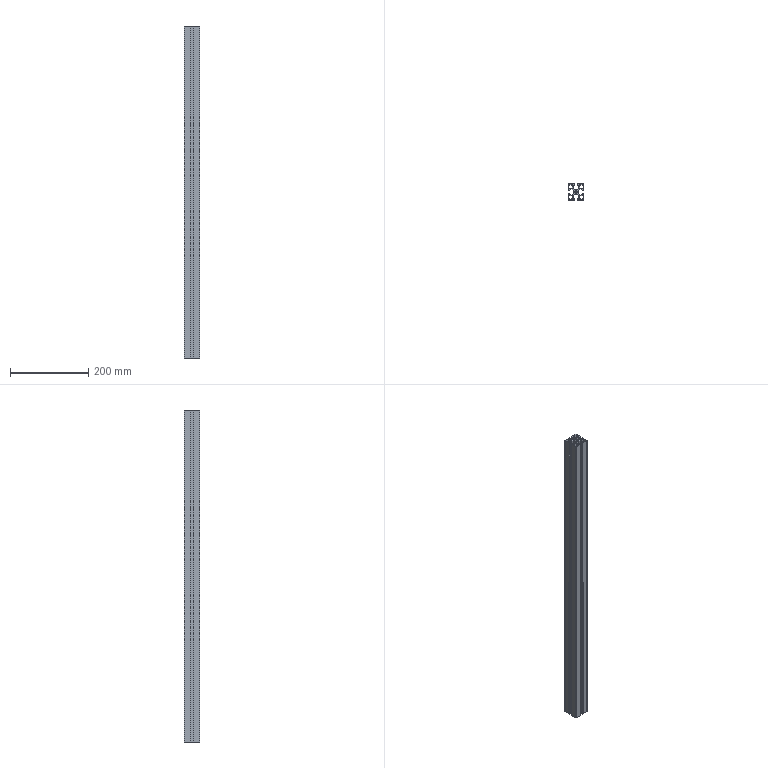Part | STEP file | 40_40_850_1-2 | 1 solid | 64 faces | box 40 x 40 x 850 mm | volume 446032 mm3 | plane 62 | cylinder 2 | commonest cylinder face diameters 6.8 x2